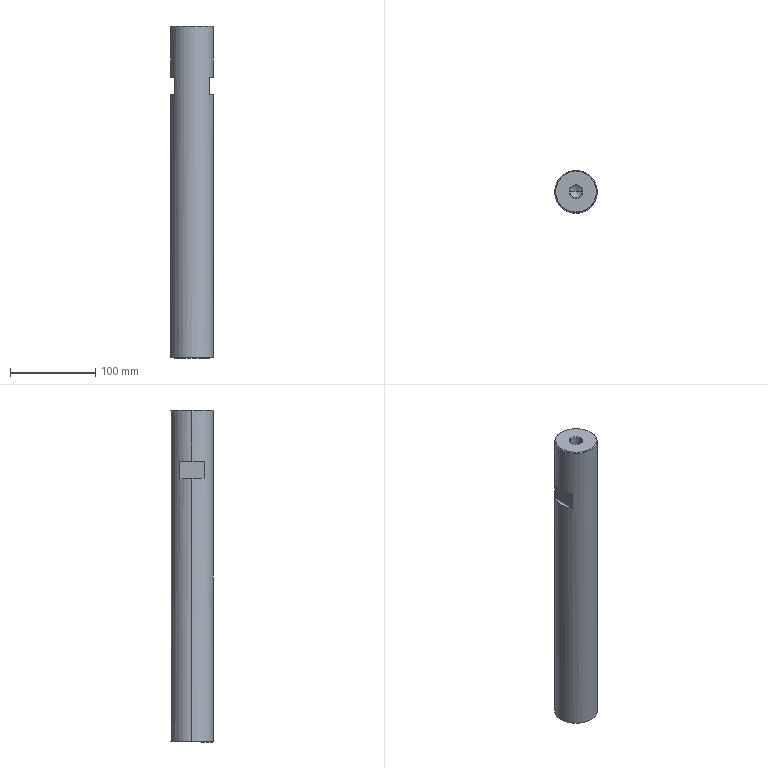Part | STEP file | SCK02-D50-L390-M16-N16-S60-Yiheda | 1 solid | 26 faces | box 50 x 50 x 390 mm | volume 752032 mm3 | cone 12 | plane 8 | cylinder 6 | commonest cylinder face diameters 13.835 x4 50 x2
STEP:
#1=CARTESIAN_POINT('',(-25.,0.,-1.));
#2=VERTEX_POINT('',#1);
#3=CARTESIAN_POINT('',(25.,0.,-1.));
#4=VERTEX_POINT('',#3);
#5=CARTESIAN_POINT('',(0.,0.,-1.));
#6=DIRECTION('',(0.,0.,-1.));
#7=DIRECTION('',(-1.,0.,0.));
#8=AXIS2_PLACEMENT_3D('',#5,#6,#7);
#9=CIRCLE('',#8,25.);
#10=EDGE_CURVE('',#2,#4,#9,.T.);
#11=ORIENTED_EDGE('',*,*,#10,.T.);
#12=CARTESIAN_POINT('',(25.,0.,-60.));
#13=VERTEX_POINT('',#12);
#14=CARTESIAN_POINT('',(25.,0.,-520.));
#15=DIRECTION('',(0.,0.,-1.));
#16=VECTOR('',#15,1000.);
#17=LINE('',#14,#16);
#18=EDGE_CURVE('',#4,#13,#17,.T.);
#19=ORIENTED_EDGE('',*,*,#18,.T.);
#20=CARTESIAN_POINT('',(20.5,14.309,-60.));
#21=VERTEX_POINT('',#20);
#22=CARTESIAN_POINT('',(0.,0.,-60.));
#23=DIRECTION('',(0.,0.,1.));
#24=DIRECTION('',(-1.,0.,0.));
#25=AXIS2_PLACEMENT_3D('',#22,#23,#24);
#26=CIRCLE('',#25,25.);
#27=EDGE_CURVE('',#13,#21,#26,.T.);
#28=ORIENTED_EDGE('',*,*,#27,.T.);
#29=CARTESIAN_POINT('',(20.5,14.309,-80.));
#30=VERTEX_POINT('',#29);
#31=CARTESIAN_POINT('',(20.5,14.309,-520.));
#32=DIRECTION('',(0.,0.,-1.));
#33=VECTOR('',#32,1000.);
#34=LINE('',#31,#33);
#35=EDGE_CURVE('',#21,#30,#34,.T.);
#36=ORIENTED_EDGE('',*,*,#35,.T.);
#37=CARTESIAN_POINT('',(25.,0.,-80.));
#38=VERTEX_POINT('',#37);
#39=CARTESIAN_POINT('',(0.,0.,-80.));
#40=DIRECTION('',(0.,0.,-1.));
#41=DIRECTION('',(-1.,0.,0.));
#42=AXIS2_PLACEMENT_3D('',#39,#40,#41);
#43=CIRCLE('',#42,25.);
#44=EDGE_CURVE('',#30,#38,#43,.T.);
#45=ORIENTED_EDGE('',*,*,#44,.T.);
#46=CARTESIAN_POINT('',(25.,0.,-389.));
#47=VERTEX_POINT('',#46);
#48=CARTESIAN_POINT('',(25.,0.,-520.));
#49=DIRECTION('',(0.,0.,-1.));
#50=VECTOR('',#49,1000.);
#51=LINE('',#48,#50);
#52=EDGE_CURVE('',#38,#47,#51,.T.);
#53=ORIENTED_EDGE('',*,*,#52,.T.);
#54=CARTESIAN_POINT('',(0.,25.,-389.));
#55=VERTEX_POINT('',#54);
#56=CARTESIAN_POINT('',(0.,0.,-389.));
#57=DIRECTION('',(0.,0.,1.));
#58=DIRECTION('',(-1.,0.,0.));
#59=AXIS2_PLACEMENT_3D('',#56,#57,#58);
#60=CIRCLE('',#59,25.);
#61=EDGE_CURVE('',#47,#55,#60,.T.);
#62=ORIENTED_EDGE('',*,*,#61,.T.);
#63=CARTESIAN_POINT('',(-25.,0.,-389.));
#64=VERTEX_POINT('',#63);
#65=CARTESIAN_POINT('',(0.,0.,-389.));
#66=DIRECTION('',(0.,0.,1.));
#67=DIRECTION('',(-1.,0.,0.));
#68=AXIS2_PLACEMENT_3D('',#65,#66,#67);
#69=CIRCLE('',#68,25.);
#70=EDGE_CURVE('',#55,#64,#69,.T.);
#71=ORIENTED_EDGE('',*,*,#70,.T.);
#72=CARTESIAN_POINT('',(-25.,0.,-80.));
#73=VERTEX_POINT('',#72);
#74=CARTESIAN_POINT('',(-25.,0.,-520.));
#75=DIRECTION('',(0.,0.,-1.));
#76=VECTOR('',#75,1000.);
#77=LINE('',#74,#76);
#78=EDGE_CURVE('',#73,#64,#77,.T.);
#79=ORIENTED_EDGE('',*,*,#78,.F.);
#80=CARTESIAN_POINT('',(-20.5,14.309,-80.));
#81=VERTEX_POINT('',#80);
#82=CARTESIAN_POINT('',(0.,0.,-80.));
#83=DIRECTION('',(0.,0.,-1.));
#84=DIRECTION('',(-1.,0.,0.));
#85=AXIS2_PLACEMENT_3D('',#82,#83,#84);
#86=CIRCLE('',#85,25.);
#87=EDGE_CURVE('',#73,#81,#86,.T.);
#88=ORIENTED_EDGE('',*,*,#87,.T.);
#89=CARTESIAN_POINT('',(-20.5,14.309,-60.));
#90=VERTEX_POINT('',#89);
#91=CARTESIAN_POINT('',(-20.5,14.309,-520.));
#92=DIRECTION('',(0.,0.,1.));
#93=VECTOR('',#92,1000.);
#94=LINE('',#91,#93);
#95=EDGE_CURVE('',#81,#90,#94,.T.);
#96=ORIENTED_EDGE('',*,*,#95,.T.);
#97=CARTESIAN_POINT('',(-25.,0.,-60.));
#98=VERTEX_POINT('',#97);
#99=CARTESIAN_POINT('',(0.,0.,-60.));
#100=DIRECTION('',(0.,0.,1.));
#101=DIRECTION('',(-1.,0.,0.));
#102=AXIS2_PLACEMENT_3D('',#99,#100,#101);
#103=CIRCLE('',#102,25.);
#104=EDGE_CURVE('',#90,#98,#103,.T.);
#105=ORIENTED_EDGE('',*,*,#104,.T.);
#106=CARTESIAN_POINT('',(-25.,0.,-520.));
#107=DIRECTION('',(0.,0.,-1.));
#108=VECTOR('',#107,1000.);
#109=LINE('',#106,#108);
#110=EDGE_CURVE('',#2,#98,#109,.T.);
#111=ORIENTED_EDGE('',*,*,#110,.F.);
#112=EDGE_LOOP('',(#11,#19,#28,#36,#45,#53,#62,#71,#79,#88,#96,#105,#111));
#113=FACE_OUTER_BOUND('',#112,.T.);
#114=CARTESIAN_POINT('',(0.,0.,-520.));
#115=DIRECTION('',(0.,0.,-1.));
#116=DIRECTION('',(-1.,0.,0.));
#117=AXIS2_PLACEMENT_3D('',#114,#115,#116);
#118=CYLINDRICAL_SURFACE('',#117,25.);
#119=ADVANCED_FACE('',(#113),#118,.T.);
#120=CARTESIAN_POINT('',(-24.,0.,0.));
#121=VERTEX_POINT('',#120);
#122=CARTESIAN_POINT('',(24.,0.,0.));
#123=VERTEX_POINT('',#122);
#124=CARTESIAN_POINT('',(0.,0.,0.));
#125=DIRECTION('',(0.,0.,-1.));
#126=DIRECTION('',(-1.,0.,0.));
#127=AXIS2_PLACEMENT_3D('',#124,#125,#126);
#128=CIRCLE('',#127,24.);
#129=EDGE_CURVE('',#121,#123,#128,.T.);
#130=ORIENTED_EDGE('',*,*,#129,.T.);
#131=CARTESIAN_POINT('',(25.,0.,-1.));
#132=DIRECTION('',(0.7071,0.,-0.7071));
#133=VECTOR('',#132,1000.);
#134=LINE('',#131,#133);
#135=EDGE_CURVE('',#123,#4,#134,.T.);
#136=ORIENTED_EDGE('',*,*,#135,.T.);
#137=ORIENTED_EDGE('',*,*,#10,.F.);
#138=CARTESIAN_POINT('',(-25.,0.,-1.));
#139=DIRECTION('',(-0.7071,0.,-0.7071));
#140=VECTOR('',#139,1000.);
#141=LINE('',#138,#140);
#142=EDGE_CURVE('',#121,#2,#141,.T.);
#143=ORIENTED_EDGE('',*,*,#142,.F.);
#144=EDGE_LOOP('',(#130,#136,#137,#143));
#145=FACE_OUTER_BOUND('',#144,.T.);
#146=CARTESIAN_POINT('',(0.,0.,-1.));
#147=DIRECTION('',(0.,0.,-1.));
#148=DIRECTION('',(-1.,0.,0.));
#149=AXIS2_PLACEMENT_3D('',#146,#147,#148);
#150=CONICAL_SURFACE('',#149,25.,0.7854);
#151=ADVANCED_FACE('',(#145),#150,.T.);
#152=CARTESIAN_POINT('',(0.,-24.,-390.));
#153=VERTEX_POINT('',#152);
#154=CARTESIAN_POINT('',(0.,24.,-390.));
#155=VERTEX_POINT('',#154);
#156=CARTESIAN_POINT('',(0.,0.,-390.));
#157=DIRECTION('',(0.,0.,1.));
#158=DIRECTION('',(0.,-1.,0.));
#159=AXIS2_PLACEMENT_3D('',#156,#157,#158);
#160=CIRCLE('',#159,24.);
#161=EDGE_CURVE('',#153,#155,#160,.T.);
#162=ORIENTED_EDGE('',*,*,#161,.T.);
#163=CARTESIAN_POINT('',(0.,25.,-389.));
#164=DIRECTION('',(0.,0.7071,0.7071));
#165=VECTOR('',#164,1000.);
#166=LINE('',#163,#165);
#167=EDGE_CURVE('',#155,#55,#166,.T.);
#168=ORIENTED_EDGE('',*,*,#167,.T.);
#169=ORIENTED_EDGE('',*,*,#61,.F.);
#170=CARTESIAN_POINT('',(0.,-25.,-389.));
#171=VERTEX_POINT('',#170);
#172=CARTESIAN_POINT('',(0.,0.,-389.));
#173=DIRECTION('',(0.,0.,1.));
#174=DIRECTION('',(-1.,0.,0.));
#175=AXIS2_PLACEMENT_3D('',#172,#173,#174);
#176=CIRCLE('',#175,25.);
#177=EDGE_CURVE('',#171,#47,#176,.T.);
#178=ORIENTED_EDGE('',*,*,#177,.F.);
#179=CARTESIAN_POINT('',(0.,-25.,-389.));
#180=DIRECTION('',(0.,-0.7071,0.7071));
#181=VECTOR('',#180,1000.);
#182=LINE('',#179,#181);
#183=EDGE_CURVE('',#153,#171,#182,.T.);
#184=ORIENTED_EDGE('',*,*,#183,.F.);
#185=EDGE_LOOP('',(#162,#168,#169,#178,#184));
#186=FACE_OUTER_BOUND('',#185,.T.);
#187=CARTESIAN_POINT('',(0.,0.,-389.));
#188=DIRECTION('',(0.,0.,1.));
#189=DIRECTION('',(0.,-1.,0.));
#190=AXIS2_PLACEMENT_3D('',#187,#188,#189);
#191=CONICAL_SURFACE('',#190,25.,0.7854);
#192=ADVANCED_FACE('',(#186),#191,.T.);
#193=CARTESIAN_POINT('',(-6.918,0.,-1.083));
#194=VERTEX_POINT('',#193);
#195=CARTESIAN_POINT('',(6.918,0.,-1.083));
#196=VERTEX_POINT('',#195);
#197=CARTESIAN_POINT('',(0.,0.,-1.083));
#198=DIRECTION('',(0.,0.,1.));
#199=DIRECTION('',(1.,0.,0.));
#200=AXIS2_PLACEMENT_3D('',#197,#198,#199);
#201=CIRCLE('',#200,6.918);
#202=EDGE_CURVE('',#194,#196,#201,.T.);
#203=ORIENTED_EDGE('',*,*,#202,.F.);
#204=CARTESIAN_POINT('',(-8.,0.,0.));
#205=VERTEX_POINT('',#204);
#206=CARTESIAN_POINT('',(-8.,0.,0.));
#207=DIRECTION('',(-0.7071,0.,0.7071));
#208=VECTOR('',#207,1000.);
#209=LINE('',#206,#208);
#210=EDGE_CURVE('',#194,#205,#209,.T.);
#211=ORIENTED_EDGE('',*,*,#210,.T.);
#212=CARTESIAN_POINT('',(8.,0.,0.));
#213=VERTEX_POINT('',#212);
#214=CARTESIAN_POINT('',(0.,0.,0.));
#215=DIRECTION('',(0.,0.,1.));
#216=DIRECTION('',(1.,0.,0.));
#217=AXIS2_PLACEMENT_3D('',#214,#215,#216);
#218=CIRCLE('',#217,8.);
#219=EDGE_CURVE('',#205,#213,#218,.T.);
#220=ORIENTED_EDGE('',*,*,#219,.T.);
#221=CARTESIAN_POINT('',(8.,0.,0.));
#222=DIRECTION('',(0.7071,0.,0.7071));
#223=VECTOR('',#222,1000.);
#224=LINE('',#221,#223);
#225=EDGE_CURVE('',#196,#213,#224,.T.);
#226=ORIENTED_EDGE('',*,*,#225,.F.);
#227=EDGE_LOOP('',(#203,#211,#220,#226));
#228=FACE_OUTER_BOUND('',#227,.T.);
#229=CARTESIAN_POINT('',(0.,0.,0.));
#230=DIRECTION('',(0.,0.,1.));
#231=DIRECTION('',(1.,0.,0.));
#232=AXIS2_PLACEMENT_3D('',#229,#230,#231);
#233=CONICAL_SURFACE('',#232,8.,0.7854);
#234=ADVANCED_FACE('',(#228),#233,.F.);
#235=CARTESIAN_POINT('',(6.917,0.,-388.918));
#236=VERTEX_POINT('',#235);
#237=CARTESIAN_POINT('',(0.,-6.917,-388.918));
#238=VERTEX_POINT('',#237);
#239=CARTESIAN_POINT('',(0.,0.,-388.918));
#240=DIRECTION('',(0.,0.,-1.));
#241=DIRECTION('',(0.,1.,0.));
#242=AXIS2_PLACEMENT_3D('',#239,#240,#241);
#243=CIRCLE('',#242,6.917);
#244=EDGE_CURVE('',#236,#238,#243,.T.);
#245=ORIENTED_EDGE('',*,*,#244,.F.);
#246=CARTESIAN_POINT('',(8.,0.,-390.));
#247=VERTEX_POINT('',#246);
#248=CARTESIAN_POINT('',(8.,0.,-390.));
#249=DIRECTION('',(0.7071,0.,-0.7071));
#250=VECTOR('',#249,1000.);
#251=LINE('',#248,#250);
#252=EDGE_CURVE('',#236,#247,#251,.T.);
#253=ORIENTED_EDGE('',*,*,#252,.T.);
#254=CARTESIAN_POINT('',(-8.,0.,-390.));
#255=VERTEX_POINT('',#254);
#256=CARTESIAN_POINT('',(0.,0.,-390.));
#257=DIRECTION('',(0.,0.,-1.));
#258=DIRECTION('',(-1.,0.,0.));
#259=AXIS2_PLACEMENT_3D('',#256,#257,#258);
#260=CIRCLE('',#259,8.);
#261=EDGE_CURVE('',#247,#255,#260,.T.);
#262=ORIENTED_EDGE('',*,*,#261,.T.);
#263=CARTESIAN_POINT('',(-6.917,0.,-388.918));
#264=VERTEX_POINT('',#263);
#265=CARTESIAN_POINT('',(-8.,0.,-390.));
#266=DIRECTION('',(-0.7071,0.,-0.7071));
#267=VECTOR('',#266,1000.);
#268=LINE('',#265,#267);
#269=EDGE_CURVE('',#264,#255,#268,.T.);
#270=ORIENTED_EDGE('',*,*,#269,.F.);
#271=CARTESIAN_POINT('',(0.,0.,-388.918));
#272=DIRECTION('',(0.,0.,-1.));
#273=DIRECTION('',(0.,1.,0.));
#274=AXIS2_PLACEMENT_3D('',#271,#272,#273);
#275=CIRCLE('',#274,6.917);
#276=EDGE_CURVE('',#238,#264,#275,.T.);
#277=ORIENTED_EDGE('',*,*,#276,.F.);
#278=EDGE_LOOP('',(#245,#253,#262,#270,#277));
#279=FACE_OUTER_BOUND('',#278,.T.);
#280=CARTESIAN_POINT('',(0.,0.,-390.));
#281=DIRECTION('',(0.,0.,-1.));
#282=DIRECTION('',(-1.,0.,0.));
#283=AXIS2_PLACEMENT_3D('',#280,#281,#282);
#284=CONICAL_SURFACE('',#283,8.,0.7854);
#285=ADVANCED_FACE('',(#279),#284,.F.);
#286=ORIENTED_EDGE('',*,*,#202,.T.);
#287=CARTESIAN_POINT('',(6.917,0.,-32.));
#288=VERTEX_POINT('',#287);
#289=CARTESIAN_POINT('',(6.918,0.,-35.994));
#290=DIRECTION('',(0.,0.,-1.));
#291=VECTOR('',#290,1000.);
#292=LINE('',#289,#291);
#293=EDGE_CURVE('',#196,#288,#292,.T.);
#294=ORIENTED_EDGE('',*,*,#293,.T.);
#295=CARTESIAN_POINT('',(-6.917,0.,-32.));
#296=VERTEX_POINT('',#295);
#297=CARTESIAN_POINT('',(0.,0.,-32.));
#298=DIRECTION('',(0.,0.,1.));
#299=DIRECTION('',(-1.,0.,0.));
#300=AXIS2_PLACEMENT_3D('',#297,#298,#299);
#301=CIRCLE('',#300,6.918);
#302=EDGE_CURVE('',#296,#288,#301,.T.);
#303=ORIENTED_EDGE('',*,*,#302,.F.);
#304=CARTESIAN_POINT('',(-6.918,0.,-35.994));
#305=DIRECTION('',(0.,0.,-1.));
#306=VECTOR('',#305,1000.);
#307=LINE('',#304,#306);
#308=EDGE_CURVE('',#194,#296,#307,.T.);
#309=ORIENTED_EDGE('',*,*,#308,.F.);
#310=EDGE_LOOP('',(#286,#294,#303,#309));
#311=FACE_OUTER_BOUND('',#310,.T.);
#312=CARTESIAN_POINT('',(0.,0.,-35.994));
#313=DIRECTION('',(0.,0.,-1.));
#314=DIRECTION('',(-1.,0.,0.));
#315=AXIS2_PLACEMENT_3D('',#312,#313,#314);
#316=CYLINDRICAL_SURFACE('',#315,6.918);
#317=ADVANCED_FACE('',(#311),#316,.F.);
#318=CARTESIAN_POINT('',(0.,-6.918,-358.));
#319=VERTEX_POINT('',#318);
#320=CARTESIAN_POINT('',(-6.918,0.,-358.));
#321=VERTEX_POINT('',#320);
#322=CARTESIAN_POINT('',(0.,0.,-358.));
#323=DIRECTION('',(0.,0.,-1.));
#324=DIRECTION('',(0.,1.,0.));
#325=AXIS2_PLACEMENT_3D('',#322,#323,#324);
#326=CIRCLE('',#325,6.918);
#327=EDGE_CURVE('',#319,#321,#326,.T.);
#328=ORIENTED_EDGE('',*,*,#327,.F.);
#329=CARTESIAN_POINT('',(0.,-6.918,-390.));
#330=DIRECTION('',(0.,0.,-1.));
#331=VECTOR('',#330,1000.);
#332=LINE('',#329,#331);
#333=EDGE_CURVE('',#319,#238,#332,.T.);
#334=ORIENTED_EDGE('',*,*,#333,.T.);
#335=ORIENTED_EDGE('',*,*,#276,.T.);
#336=CARTESIAN_POINT('',(0.,6.917,-388.918));
#337=VERTEX_POINT('',#336);
#338=CARTESIAN_POINT('',(0.,0.,-388.918));
#339=DIRECTION('',(0.,0.,-1.));
#340=DIRECTION('',(0.,1.,0.));
#341=AXIS2_PLACEMENT_3D('',#338,#339,#340);
#342=CIRCLE('',#341,6.917);
#343=EDGE_CURVE('',#264,#337,#342,.T.);
#344=ORIENTED_EDGE('',*,*,#343,.T.);
#345=CARTESIAN_POINT('',(0.,6.918,-358.));
#346=VERTEX_POINT('',#345);
#347=CARTESIAN_POINT('',(0.,6.918,-390.));
#348=DIRECTION('',(0.,0.,-1.));
#349=VECTOR('',#348,1000.);
#350=LINE('',#347,#349);
#351=EDGE_CURVE('',#346,#337,#350,.T.);
#352=ORIENTED_EDGE('',*,*,#351,.F.);
#353=CARTESIAN_POINT('',(0.,0.,-358.));
#354=DIRECTION('',(0.,0.,-1.));
#355=DIRECTION('',(0.,1.,0.));
#356=AXIS2_PLACEMENT_3D('',#353,#354,#355);
#357=CIRCLE('',#356,6.918);
#358=EDGE_CURVE('',#321,#346,#357,.T.);
#359=ORIENTED_EDGE('',*,*,#358,.F.);
#360=EDGE_LOOP('',(#328,#334,#335,#344,#352,#359));
#361=FACE_OUTER_BOUND('',#360,.T.);
#362=CARTESIAN_POINT('',(0.,0.,-390.));
#363=DIRECTION('',(0.,0.,-1.));
#364=DIRECTION('',(0.,1.,0.));
#365=AXIS2_PLACEMENT_3D('',#362,#363,#364);
#366=CYLINDRICAL_SURFACE('',#365,6.918);
#367=ADVANCED_FACE('',(#361),#366,.F.);
#368=CARTESIAN_POINT('',(0.,0.,-35.994));
#369=VERTEX_POINT('',#368);
#370=CARTESIAN_POINT('',(6.917,0.,-32.));
#371=DIRECTION('',(0.866,0.,0.5));
#372=VECTOR('',#371,1000.);
#373=LINE('',#370,#372);
#374=EDGE_CURVE('',#369,#288,#373,.T.);
#375=ORIENTED_EDGE('',*,*,#374,.F.);
#376=CARTESIAN_POINT('',(-6.917,0.,-32.));
#377=DIRECTION('',(-0.866,0.,0.5));
#378=VECTOR('',#377,1000.);
#379=LINE('',#376,#378);
#380=EDGE_CURVE('',#369,#296,#379,.T.);
#381=ORIENTED_EDGE('',*,*,#380,.T.);
#382=ORIENTED_EDGE('',*,*,#302,.T.);
#383=EDGE_LOOP('',(#375,#381,#382));
#384=FACE_OUTER_BOUND('',#383,.T.);
#385=CARTESIAN_POINT('',(0.,0.,-32.));
#386=DIRECTION('',(0.,0.,1.));
#387=DIRECTION('',(1.,0.,0.));
#388=AXIS2_PLACEMENT_3D('',#385,#386,#387);
#389=CONICAL_SURFACE('',#388,6.917,1.047);
#390=ADVANCED_FACE('',(#384),#389,.F.);
#391=CARTESIAN_POINT('',(0.,0.,-354.006));
#392=VERTEX_POINT('',#391);
#393=CARTESIAN_POINT('',(-6.917,0.,-358.));
#394=DIRECTION('',(-0.866,0.,-0.5));
#395=VECTOR('',#394,1000.);
#396=LINE('',#393,#395);
#397=EDGE_CURVE('',#392,#321,#396,.T.);
#398=ORIENTED_EDGE('',*,*,#397,.F.);
#399=CARTESIAN_POINT('',(6.918,0.,-358.));
#400=VERTEX_POINT('',#399);
#401=CARTESIAN_POINT('',(6.917,0.,-358.));
#402=DIRECTION('',(0.866,0.,-0.5));
#403=VECTOR('',#402,1000.);
#404=LINE('',#401,#403);
#405=EDGE_CURVE('',#392,#400,#404,.T.);
#406=ORIENTED_EDGE('',*,*,#405,.T.);
#407=CARTESIAN_POINT('',(0.,0.,-358.));
#408=DIRECTION('',(0.,0.,-1.));
#409=DIRECTION('',(0.,1.,0.));
#410=AXIS2_PLACEMENT_3D('',#407,#408,#409);
#411=CIRCLE('',#410,6.918);
#412=EDGE_CURVE('',#400,#319,#411,.T.);
#413=ORIENTED_EDGE('',*,*,#412,.T.);
#414=ORIENTED_EDGE('',*,*,#327,.T.);
#415=EDGE_LOOP('',(#398,#406,#413,#414));
#416=FACE_OUTER_BOUND('',#415,.T.);
#417=CARTESIAN_POINT('',(0.,0.,-358.));
#418=DIRECTION('',(0.,0.,-1.));
#419=DIRECTION('',(-1.,0.,0.));
#420=AXIS2_PLACEMENT_3D('',#417,#418,#419);
#421=CONICAL_SURFACE('',#420,6.917,1.047);
#422=ADVANCED_FACE('',(#416),#421,.F.);
#423=ORIENTED_EDGE('',*,*,#18,.F.);
#424=CARTESIAN_POINT('',(0.,0.,-1.));
#425=DIRECTION('',(0.,0.,-1.));
#426=DIRECTION('',(-1.,0.,0.));
#427=AXIS2_PLACEMENT_3D('',#424,#425,#426);
#428=CIRCLE('',#427,25.);
#429=EDGE_CURVE('',#4,#2,#428,.T.);
#430=ORIENTED_EDGE('',*,*,#429,.T.);
#431=ORIENTED_EDGE('',*,*,#110,.T.);
#432=CARTESIAN_POINT('',(-20.5,-14.309,-60.));
#433=VERTEX_POINT('',#432);
#434=CARTESIAN_POINT('',(0.,0.,-60.));
#435=DIRECTION('',(0.,0.,1.));
#436=DIRECTION('',(-1.,0.,0.));
#437=AXIS2_PLACEMENT_3D('',#434,#435,#436);
#438=CIRCLE('',#437,25.);
#439=EDGE_CURVE('',#98,#433,#438,.T.);
#440=ORIENTED_EDGE('',*,*,#439,.T.);
#441=CARTESIAN_POINT('',(-20.5,-14.309,-80.));
#442=VERTEX_POINT('',#441);
#443=CARTESIAN_POINT('',(-20.5,-14.309,-520.));
#444=DIRECTION('',(0.,0.,-1.));
#445=VECTOR('',#444,1000.);
#446=LINE('',#443,#445);
#447=EDGE_CURVE('',#433,#442,#446,.T.);
#448=ORIENTED_EDGE('',*,*,#447,.T.);
#449=CARTESIAN_POINT('',(0.,0.,-80.));
#450=DIRECTION('',(0.,0.,-1.));
#451=DIRECTION('',(-1.,0.,0.));
#452=AXIS2_PLACEMENT_3D('',#449,#450,#451);
#453=CIRCLE('',#452,25.);
#454=EDGE_CURVE('',#442,#73,#453,.T.);
#455=ORIENTED_EDGE('',*,*,#454,.T.);
#456=ORIENTED_EDGE('',*,*,#78,.T.);
#457=CARTESIAN_POINT('',(0.,0.,-389.));
#458=DIRECTION('',(0.,0.,1.));
#459=DIRECTION('',(-1.,0.,0.));
#460=AXIS2_PLACEMENT_3D('',#457,#458,#459);
#461=CIRCLE('',#460,25.);
#462=EDGE_CURVE('',#64,#171,#461,.T.);
#463=ORIENTED_EDGE('',*,*,#462,.T.);
#464=ORIENTED_EDGE('',*,*,#177,.T.);
#465=ORIENTED_EDGE('',*,*,#52,.F.);
#466=CARTESIAN_POINT('',(20.5,-14.309,-80.));
#467=VERTEX_POINT('',#466);
#468=CARTESIAN_POINT('',(0.,0.,-80.));
#469=DIRECTION('',(0.,0.,-1.));
#470=DIRECTION('',(-1.,0.,0.));
#471=AXIS2_PLACEMENT_3D('',#468,#469,#470);
#472=CIRCLE('',#471,25.);
#473=EDGE_CURVE('',#38,#467,#472,.T.);
#474=ORIENTED_EDGE('',*,*,#473,.T.);
#475=CARTESIAN_POINT('',(20.5,-14.309,-60.));
#476=VERTEX_POINT('',#475);
#477=CARTESIAN_POINT('',(20.5,-14.309,-520.));
#478=DIRECTION('',(0.,0.,1.));
#479=VECTOR('',#478,1000.);
#480=LINE('',#477,#479);
#481=EDGE_CURVE('',#467,#476,#480,.T.);
#482=ORIENTED_EDGE('',*,*,#481,.T.);
#483=CARTESIAN_POINT('',(0.,0.,-60.));
#484=DIRECTION('',(0.,0.,1.));
#485=DIRECTION('',(-1.,0.,0.));
#486=AXIS2_PLACEMENT_3D('',#483,#484,#485);
#487=CIRCLE('',#486,25.);
#488=EDGE_CURVE('',#476,#13,#487,.T.);
#489=ORIENTED_EDGE('',*,*,#488,.T.);
#490=EDGE_LOOP('',(#423,#430,#431,#440,#448,#455,#456,#463,#464,#465,#474,#482,#489));
#491=FACE_OUTER_BOUND('',#490,.T.);
#492=CARTESIAN_POINT('',(0.,0.,-520.));
#493=DIRECTION('',(0.,0.,-1.));
#494=DIRECTION('',(-1.,0.,0.));
#495=AXIS2_PLACEMENT_3D('',#492,#493,#494);
#496=CYLINDRICAL_SURFACE('',#495,25.);
#497=ADVANCED_FACE('',(#491),#496,.T.);
#498=CARTESIAN_POINT('',(20.5,-14.309,-80.));
#499=DIRECTION('',(0.,1.,0.));
#500=VECTOR('',#499,1000.);
#501=LINE('',#498,#500);
#502=EDGE_CURVE('',#467,#30,#501,.T.);
#503=ORIENTED_EDGE('',*,*,#502,.T.);
#504=ORIENTED_EDGE('',*,*,#35,.F.);
#505=CARTESIAN_POINT('',(20.5,-14.309,-60.));
#506=DIRECTION('',(0.,-1.,0.));
#507=VECTOR('',#506,1000.);
#508=LINE('',#505,#507);
#509=EDGE_CURVE('',#21,#476,#508,.T.);
#510=ORIENTED_EDGE('',*,*,#509,.T.);
#511=ORIENTED_EDGE('',*,*,#481,.F.);
#512=EDGE_LOOP('',(#503,#504,#510,#511));
#513=FACE_OUTER_BOUND('',#512,.T.);
#514=CARTESIAN_POINT('',(20.5,-14.309,-80.));
#515=DIRECTION('',(1.,0.,0.));
#516=DIRECTION('',(0.,0.,-1.));
#517=AXIS2_PLACEMENT_3D('',#514,#515,#516);
#518=PLANE('',#517);
#519=ADVANCED_FACE('',(#513),#518,.T.);
#520=ORIENTED_EDGE('',*,*,#44,.F.);
#521=ORIENTED_EDGE('',*,*,#502,.F.);
#522=ORIENTED_EDGE('',*,*,#473,.F.);
#523=EDGE_LOOP('',(#520,#521,#522));
#524=FACE_OUTER_BOUND('',#523,.T.);
#525=CARTESIAN_POINT('',(0.,0.,-80.));
#526=DIRECTION('',(0.,0.,1.));
#527=DIRECTION('',(1.,0.,0.));
#528=AXIS2_PLACEMENT_3D('',#525,#526,#527);
#529=PLANE('',#528);
#530=ADVANCED_FACE('',(#524),#529,.T.);
#531=ORIENTED_EDGE('',*,*,#488,.F.);
#532=ORIENTED_EDGE('',*,*,#509,.F.);
#533=ORIENTED_EDGE('',*,*,#27,.F.);
#534=EDGE_LOOP('',(#531,#532,#533));
#535=FACE_OUTER_BOUND('',#534,.T.);
#536=CARTESIAN_POINT('',(0.,0.,-60.));
#537=DIRECTION('',(0.,0.,1.));
#538=DIRECTION('',(1.,0.,0.));
#539=AXIS2_PLACEMENT_3D('',#536,#537,#538);
#540=PLANE('',#539);
#541=ADVANCED_FACE('',(#535),#540,.F.);
#542=CARTESIAN_POINT('',(-20.5,14.309,-80.));
#543=DIRECTION('',(0.,-1.,0.));
#544=VECTOR('',#543,1000.);
#545=LINE('',#542,#544);
#546=EDGE_CURVE('',#81,#442,#545,.T.);
#547=ORIENTED_EDGE('',*,*,#546,.T.);
#548=ORIENTED_EDGE('',*,*,#447,.F.);
#549=CARTESIAN_POINT('',(-20.5,14.309,-60.));
#550=DIRECTION('',(0.,1.,0.));
#551=VECTOR('',#550,1000.);
#552=LINE('',#549,#551);
#553=EDGE_CURVE('',#433,#90,#552,.T.);
#554=ORIENTED_EDGE('',*,*,#553,.T.);
#555=ORIENTED_EDGE('',*,*,#95,.F.);
#556=EDGE_LOOP('',(#547,#548,#554,#555));
#557=FACE_OUTER_BOUND('',#556,.T.);
#558=CARTESIAN_POINT('',(-20.5,14.309,-80.));
#559=DIRECTION('',(-1.,0.,0.));
#560=DIRECTION('',(0.,0.,1.));
#561=AXIS2_PLACEMENT_3D('',#558,#559,#560);
#562=PLANE('',#561);
#563=ADVANCED_FACE('',(#557),#562,.T.);
#564=ORIENTED_EDGE('',*,*,#104,.F.);
#565=ORIENTED_EDGE('',*,*,#553,.F.);
#566=ORIENTED_EDGE('',*,*,#439,.F.);
#567=EDGE_LOOP('',(#564,#565,#566));
#568=FACE_OUTER_BOUND('',#567,.T.);
#569=CARTESIAN_POINT('',(0.,0.,-60.));
#570=DIRECTION('',(0.,0.,1.));
#571=DIRECTION('',(1.,0.,0.));
#572=AXIS2_PLACEMENT_3D('',#569,#570,#571);
#573=PLANE('',#572);
#574=ADVANCED_FACE('',(#568),#573,.F.);
#575=ORIENTED_EDGE('',*,*,#454,.F.);
#576=ORIENTED_EDGE('',*,*,#546,.F.);
#577=ORIENTED_EDGE('',*,*,#87,.F.);
#578=EDGE_LOOP('',(#575,#576,#577));
#579=FACE_OUTER_BOUND('',#578,.T.);
#580=CARTESIAN_POINT('',(0.,0.,-80.));
#581=DIRECTION('',(0.,0.,1.));
#582=DIRECTION('',(1.,0.,0.));
#583=AXIS2_PLACEMENT_3D('',#580,#581,#582);
#584=PLANE('',#583);
#585=ADVANCED_FACE('',(#579),#584,.T.);
#586=ORIENTED_EDGE('',*,*,#135,.F.);
#587=CARTESIAN_POINT('',(0.,0.,0.));
#588=DIRECTION('',(0.,0.,-1.));
#589=DIRECTION('',(-1.,0.,0.));
#590=AXIS2_PLACEMENT_3D('',#587,#588,#589);
#591=CIRCLE('',#590,24.);
#592=EDGE_CURVE('',#123,#121,#591,.T.);
#593=ORIENTED_EDGE('',*,*,#592,.T.);
#594=ORIENTED_EDGE('',*,*,#142,.T.);
#595=ORIENTED_EDGE('',*,*,#429,.F.);
#596=EDGE_LOOP('',(#586,#593,#594,#595));
#597=FACE_OUTER_BOUND('',#596,.T.);
#598=CARTESIAN_POINT('',(0.,0.,-1.));
#599=DIRECTION('',(0.,0.,-1.));
#600=DIRECTION('',(-1.,0.,0.));
#601=AXIS2_PLACEMENT_3D('',#598,#599,#600);
#602=CONICAL_SURFACE('',#601,25.,0.7854);
#603=ADVANCED_FACE('',(#597),#602,.T.);
#604=ORIENTED_EDGE('',*,*,#167,.F.);
#605=CARTESIAN_POINT('',(0.,0.,-390.));
#606=DIRECTION('',(0.,0.,1.));
#607=DIRECTION('',(0.,-1.,0.));
#608=AXIS2_PLACEMENT_3D('',#605,#606,#607);
#609=CIRCLE('',#608,24.);
#610=EDGE_CURVE('',#155,#153,#609,.T.);
#611=ORIENTED_EDGE('',*,*,#610,.T.);
#612=ORIENTED_EDGE('',*,*,#183,.T.);
#613=ORIENTED_EDGE('',*,*,#462,.F.);
#614=ORIENTED_EDGE('',*,*,#70,.F.);
#615=EDGE_LOOP('',(#604,#611,#612,#613,#614));
#616=FACE_OUTER_BOUND('',#615,.T.);
#617=CARTESIAN_POINT('',(0.,0.,-389.));
#618=DIRECTION('',(0.,0.,1.));
#619=DIRECTION('',(0.,-1.,0.));
#620=AXIS2_PLACEMENT_3D('',#617,#618,#619);
#621=CONICAL_SURFACE('',#620,25.,0.7854);
#622=ADVANCED_FACE('',(#616),#621,.T.);
#623=CARTESIAN_POINT('',(0.,0.,0.));
#624=DIRECTION('',(0.,0.,1.));
#625=DIRECTION('',(1.,0.,0.));
#626=AXIS2_PLACEMENT_3D('',#623,#624,#625);
#627=CIRCLE('',#626,8.);
#628=EDGE_CURVE('',#213,#205,#627,.T.);
#629=ORIENTED_EDGE('',*,*,#628,.F.);
#630=ORIENTED_EDGE('',*,*,#219,.F.);
#631=EDGE_LOOP('',(#629,#630));
#632=FACE_BOUND('',#631,.T.);
#633=ORIENTED_EDGE('',*,*,#129,.F.);
#634=ORIENTED_EDGE('',*,*,#592,.F.);
#635=EDGE_LOOP('',(#633,#634));
#636=FACE_OUTER_BOUND('',#635,.T.);
#637=CARTESIAN_POINT('',(0.,0.,0.));
#638=DIRECTION('',(0.,0.,-1.));
#639=DIRECTION('',(-1.,0.,0.));
#640=AXIS2_PLACEMENT_3D('',#637,#638,#639);
#641=PLANE('',#640);
#642=ADVANCED_FACE('',(#632,#636),#641,.F.);
#643=ORIENTED_EDGE('',*,*,#161,.F.);
#644=ORIENTED_EDGE('',*,*,#610,.F.);
#645=EDGE_LOOP('',(#643,#644));
#646=FACE_OUTER_BOUND('',#645,.T.);
#647=CARTESIAN_POINT('',(0.,0.,-390.));
#648=DIRECTION('',(0.,0.,-1.));
#649=DIRECTION('',(-1.,0.,0.));
#650=AXIS2_PLACEMENT_3D('',#647,#648,#649);
#651=CIRCLE('',#650,8.);
#652=EDGE_CURVE('',#255,#247,#651,.T.);
#653=ORIENTED_EDGE('',*,*,#652,.F.);
#654=ORIENTED_EDGE('',*,*,#261,.F.);
#655=EDGE_LOOP('',(#653,#654));
#656=FACE_BOUND('',#655,.T.);
#657=CARTESIAN_POINT('',(0.,24.,-390.));
#658=DIRECTION('',(0.,0.,1.));
#659=DIRECTION('',(1.,0.,0.));
#660=AXIS2_PLACEMENT_3D('',#657,#658,#659);
#661=PLANE('',#660);
#662=ADVANCED_FACE('',(#646,#656),#661,.F.);
#663=ORIENTED_EDGE('',*,*,#210,.F.);
#664=CARTESIAN_POINT('',(0.,0.,-1.083));
#665=DIRECTION('',(0.,0.,1.));
#666=DIRECTION('',(1.,0.,0.));
#667=AXIS2_PLACEMENT_3D('',#664,#665,#666);
#668=CIRCLE('',#667,6.918);
#669=EDGE_CURVE('',#196,#194,#668,.T.);
#670=ORIENTED_EDGE('',*,*,#669,.F.);
#671=ORIENTED_EDGE('',*,*,#225,.T.);
#672=ORIENTED_EDGE('',*,*,#628,.T.);
#673=EDGE_LOOP('',(#663,#670,#671,#672));
#674=FACE_OUTER_BOUND('',#673,.T.);
#675=CARTESIAN_POINT('',(0.,0.,0.));
#676=DIRECTION('',(0.,0.,1.));
#677=DIRECTION('',(1.,0.,0.));
#678=AXIS2_PLACEMENT_3D('',#675,#676,#677);
#679=CONICAL_SURFACE('',#678,8.,0.7854);
#680=ADVANCED_FACE('',(#674),#679,.F.);
#681=ORIENTED_EDGE('',*,*,#252,.F.);
#682=CARTESIAN_POINT('',(0.,0.,-388.918));
#683=DIRECTION('',(0.,0.,-1.));
#684=DIRECTION('',(0.,1.,0.));
#685=AXIS2_PLACEMENT_3D('',#682,#683,#684);
#686=CIRCLE('',#685,6.917);
#687=EDGE_CURVE('',#337,#236,#686,.T.);
#688=ORIENTED_EDGE('',*,*,#687,.F.);
#689=ORIENTED_EDGE('',*,*,#343,.F.);
#690=ORIENTED_EDGE('',*,*,#269,.T.);
#691=ORIENTED_EDGE('',*,*,#652,.T.);
#692=EDGE_LOOP('',(#681,#688,#689,#690,#691));
#693=FACE_OUTER_BOUND('',#692,.T.);
#694=CARTESIAN_POINT('',(0.,0.,-390.));
#695=DIRECTION('',(0.,0.,-1.));
#696=DIRECTION('',(-1.,0.,0.));
#697=AXIS2_PLACEMENT_3D('',#694,#695,#696);
#698=CONICAL_SURFACE('',#697,8.,0.7854);
#699=ADVANCED_FACE('',(#693),#698,.F.);
#700=ORIENTED_EDGE('',*,*,#293,.F.);
#701=ORIENTED_EDGE('',*,*,#669,.T.);
#702=ORIENTED_EDGE('',*,*,#308,.T.);
#703=CARTESIAN_POINT('',(0.,0.,-32.));
#704=DIRECTION('',(0.,0.,1.));
#705=DIRECTION('',(-1.,0.,0.));
#706=AXIS2_PLACEMENT_3D('',#703,#704,#705);
#707=CIRCLE('',#706,6.918);
#708=EDGE_CURVE('',#288,#296,#707,.T.);
#709=ORIENTED_EDGE('',*,*,#708,.F.);
#710=EDGE_LOOP('',(#700,#701,#702,#709));
#711=FACE_OUTER_BOUND('',#710,.T.);
#712=CARTESIAN_POINT('',(0.,0.,-35.994));
#713=DIRECTION('',(0.,0.,-1.));
#714=DIRECTION('',(-1.,0.,0.));
#715=AXIS2_PLACEMENT_3D('',#712,#713,#714);
#716=CYLINDRICAL_SURFACE('',#715,6.918);
#717=ADVANCED_FACE('',(#711),#716,.F.);
#718=ORIENTED_EDGE('',*,*,#333,.F.);
#719=ORIENTED_EDGE('',*,*,#412,.F.);
#720=CARTESIAN_POINT('',(0.,0.,-358.));
#721=DIRECTION('',(0.,0.,-1.));
#722=DIRECTION('',(0.,1.,0.));
#723=AXIS2_PLACEMENT_3D('',#720,#721,#722);
#724=CIRCLE('',#723,6.918);
#725=EDGE_CURVE('',#346,#400,#724,.T.);
#726=ORIENTED_EDGE('',*,*,#725,.F.);
#727=ORIENTED_EDGE('',*,*,#351,.T.);
#728=ORIENTED_EDGE('',*,*,#687,.T.);
#729=ORIENTED_EDGE('',*,*,#244,.T.);
#730=EDGE_LOOP('',(#718,#719,#726,#727,#728,#729));
#731=FACE_OUTER_BOUND('',#730,.T.);
#732=CARTESIAN_POINT('',(0.,0.,-390.));
#733=DIRECTION('',(0.,0.,-1.));
#734=DIRECTION('',(0.,1.,0.));
#735=AXIS2_PLACEMENT_3D('',#732,#733,#734);
#736=CYLINDRICAL_SURFACE('',#735,6.918);
#737=ADVANCED_FACE('',(#731),#736,.F.);
#738=ORIENTED_EDGE('',*,*,#380,.F.);
#739=ORIENTED_EDGE('',*,*,#374,.T.);
#740=ORIENTED_EDGE('',*,*,#708,.T.);
#741=EDGE_LOOP('',(#738,#739,#740));
#742=FACE_OUTER_BOUND('',#741,.T.);
#743=CARTESIAN_POINT('',(0.,0.,-32.));
#744=DIRECTION('',(0.,0.,1.));
#745=DIRECTION('',(1.,0.,0.));
#746=AXIS2_PLACEMENT_3D('',#743,#744,#745);
#747=CONICAL_SURFACE('',#746,6.917,1.047);
#748=ADVANCED_FACE('',(#742),#747,.F.);
#749=ORIENTED_EDGE('',*,*,#405,.F.);
#750=ORIENTED_EDGE('',*,*,#397,.T.);
#751=ORIENTED_EDGE('',*,*,#358,.T.);
#752=ORIENTED_EDGE('',*,*,#725,.T.);
#753=EDGE_LOOP('',(#749,#750,#751,#752));
#754=FACE_OUTER_BOUND('',#753,.T.);
#755=CARTESIAN_POINT('',(0.,0.,-358.));
#756=DIRECTION('',(0.,0.,-1.));
#757=DIRECTION('',(-1.,0.,0.));
#758=AXIS2_PLACEMENT_3D('',#755,#756,#757);
#759=CONICAL_SURFACE('',#758,6.917,1.047);
#760=ADVANCED_FACE('',(#754),#759,.F.);
#761=CLOSED_SHELL('',(#119,#151,#192,#234,#285,#317,#367,#390,#422,#497,#519,#530,#541,#563,#574,#585,#603,#622,#642,#662,#680,#699,#717,#737,#748,#760));
#762=MANIFOLD_SOLID_BREP('',#761);
#763=CARTESIAN_POINT('',(0.,0.,0.));
#764=DIRECTION('',(0.,0.,1.));
#765=DIRECTION('',(1.,0.,0.));
#766=AXIS2_PLACEMENT_3D('',#763,#764,#765);
#767=(LENGTH_UNIT()NAMED_UNIT(*)SI_UNIT(.MILLI.,.METRE.));
#768=UNCERTAINTY_MEASURE_WITH_UNIT(LENGTH_MEASURE(0.00001),#767,'','');
#769=(NAMED_UNIT(*)PLANE_ANGLE_UNIT()SI_UNIT($,.RADIAN.));
#770=(NAMED_UNIT(*)SI_UNIT($,.STERADIAN.)SOLID_ANGLE_UNIT());
#771=(GEOMETRIC_REPRESENTATION_CONTEXT(3)GLOBAL_UNCERTAINTY_ASSIGNED_CONTEXT((#768))GLOBAL_UNIT_ASSIGNED_CONTEXT((#767,#769,#770))REPRESENTATION_CONTEXT('',''));
#772=ADVANCED_BREP_SHAPE_REPRESENTATION('',(#762,#766),#771);